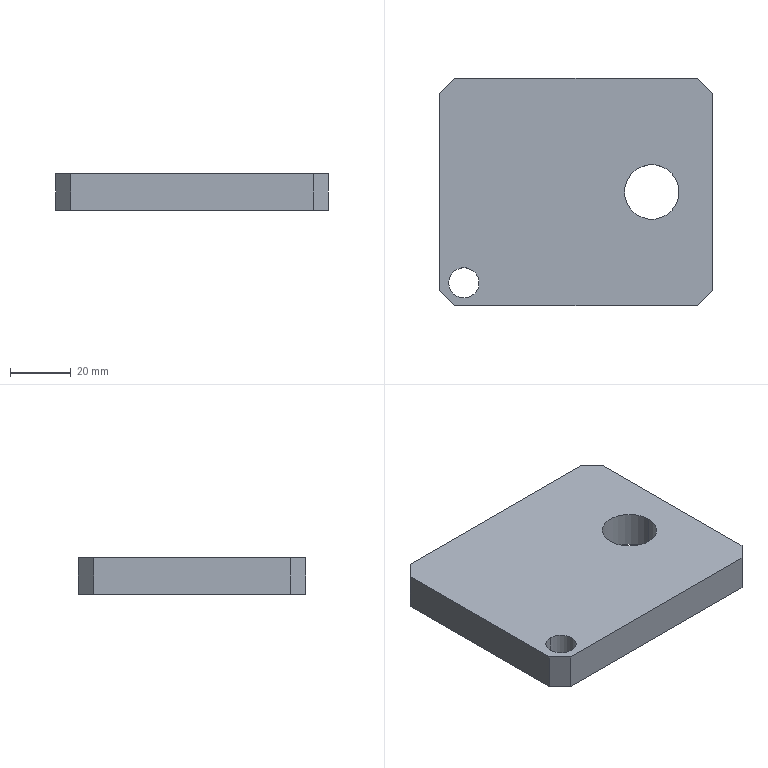Part | STEP file | [17] | 1 solid | 14 faces | box 90 x 75 x 12 mm | volume 76404 mm3 | plane 10 | cylinder 4 | commonest cylinder face diameters 10 x2 18 x2
STEP:
#1=CARTESIAN_POINT('',(79.,37.5,0.));
#2=VERTEX_POINT('',#1);
#3=CARTESIAN_POINT('',(61.,37.5,0.));
#4=VERTEX_POINT('',#3);
#5=CARTESIAN_POINT('',(70.,37.5,0.));
#6=DIRECTION('',(0.,0.,1.));
#7=DIRECTION('',(-1.,0.,0.));
#8=AXIS2_PLACEMENT_3D('',#5,#6,#7);
#9=CIRCLE('',#8,9.);
#10=EDGE_CURVE('',#2,#4,#9,.T.);
#11=ORIENTED_EDGE('',*,*,#10,.F.);
#12=CARTESIAN_POINT('',(79.,37.5,12.));
#13=VERTEX_POINT('',#12);
#14=CARTESIAN_POINT('',(79.,37.5,0.));
#15=DIRECTION('',(0.,0.,1.));
#16=VECTOR('',#15,1000.);
#17=LINE('',#14,#16);
#18=EDGE_CURVE('',#2,#13,#17,.T.);
#19=ORIENTED_EDGE('',*,*,#18,.T.);
#20=CARTESIAN_POINT('',(61.,37.5,12.));
#21=VERTEX_POINT('',#20);
#22=CARTESIAN_POINT('',(70.,37.5,12.));
#23=DIRECTION('',(0.,0.,-1.));
#24=DIRECTION('',(1.,0.,0.));
#25=AXIS2_PLACEMENT_3D('',#22,#23,#24);
#26=CIRCLE('',#25,9.);
#27=EDGE_CURVE('',#21,#13,#26,.T.);
#28=ORIENTED_EDGE('',*,*,#27,.F.);
#29=CARTESIAN_POINT('',(61.,37.5,0.));
#30=DIRECTION('',(0.,0.,1.));
#31=VECTOR('',#30,1000.);
#32=LINE('',#29,#31);
#33=EDGE_CURVE('',#4,#21,#32,.T.);
#34=ORIENTED_EDGE('',*,*,#33,.F.);
#35=EDGE_LOOP('',(#11,#19,#28,#34));
#36=FACE_OUTER_BOUND('',#35,.T.);
#37=CARTESIAN_POINT('',(70.,37.5,0.));
#38=DIRECTION('',(0.,0.,1.));
#39=DIRECTION('',(-1.,0.,0.));
#40=AXIS2_PLACEMENT_3D('',#37,#38,#39);
#41=CYLINDRICAL_SURFACE('',#40,9.);
#42=ADVANCED_FACE('',(#36),#41,.F.);
#43=CARTESIAN_POINT('',(8.,2.5,12.));
#44=VERTEX_POINT('',#43);
#45=CARTESIAN_POINT('',(8.,12.5,12.));
#46=VERTEX_POINT('',#45);
#47=CARTESIAN_POINT('',(8.,7.5,12.));
#48=DIRECTION('',(0.,0.,-1.));
#49=DIRECTION('',(0.,1.,0.));
#50=AXIS2_PLACEMENT_3D('',#47,#48,#49);
#51=CIRCLE('',#50,5.);
#52=EDGE_CURVE('',#44,#46,#51,.T.);
#53=ORIENTED_EDGE('',*,*,#52,.F.);
#54=CARTESIAN_POINT('',(8.,2.5,0.));
#55=VERTEX_POINT('',#54);
#56=CARTESIAN_POINT('',(8.,2.5,12.));
#57=DIRECTION('',(0.,0.,-1.));
#58=VECTOR('',#57,1000.);
#59=LINE('',#56,#58);
#60=EDGE_CURVE('',#44,#55,#59,.T.);
#61=ORIENTED_EDGE('',*,*,#60,.T.);
#62=CARTESIAN_POINT('',(8.,12.5,0.));
#63=VERTEX_POINT('',#62);
#64=CARTESIAN_POINT('',(8.,7.5,0.));
#65=DIRECTION('',(0.,0.,1.));
#66=DIRECTION('',(0.,-1.,0.));
#67=AXIS2_PLACEMENT_3D('',#64,#65,#66);
#68=CIRCLE('',#67,5.);
#69=EDGE_CURVE('',#63,#55,#68,.T.);
#70=ORIENTED_EDGE('',*,*,#69,.F.);
#71=CARTESIAN_POINT('',(8.,12.5,12.));
#72=DIRECTION('',(0.,0.,-1.));
#73=VECTOR('',#72,1000.);
#74=LINE('',#71,#73);
#75=EDGE_CURVE('',#46,#63,#74,.T.);
#76=ORIENTED_EDGE('',*,*,#75,.F.);
#77=EDGE_LOOP('',(#53,#61,#70,#76));
#78=FACE_OUTER_BOUND('',#77,.T.);
#79=CARTESIAN_POINT('',(8.,7.5,12.));
#80=DIRECTION('',(0.,0.,-1.));
#81=DIRECTION('',(0.,1.,0.));
#82=AXIS2_PLACEMENT_3D('',#79,#80,#81);
#83=CYLINDRICAL_SURFACE('',#82,5.);
#84=ADVANCED_FACE('',(#78),#83,.F.);
#85=CARTESIAN_POINT('',(70.,37.5,0.));
#86=DIRECTION('',(0.,0.,1.));
#87=DIRECTION('',(-1.,0.,0.));
#88=AXIS2_PLACEMENT_3D('',#85,#86,#87);
#89=CIRCLE('',#88,9.);
#90=EDGE_CURVE('',#4,#2,#89,.T.);
#91=ORIENTED_EDGE('',*,*,#90,.T.);
#92=ORIENTED_EDGE('',*,*,#10,.T.);
#93=EDGE_LOOP('',(#91,#92));
#94=FACE_BOUND('',#93,.T.);
#95=ORIENTED_EDGE('',*,*,#69,.T.);
#96=CARTESIAN_POINT('',(8.,7.5,0.));
#97=DIRECTION('',(0.,0.,1.));
#98=DIRECTION('',(0.,-1.,0.));
#99=AXIS2_PLACEMENT_3D('',#96,#97,#98);
#100=CIRCLE('',#99,5.);
#101=EDGE_CURVE('',#55,#63,#100,.T.);
#102=ORIENTED_EDGE('',*,*,#101,.T.);
#103=EDGE_LOOP('',(#95,#102));
#104=FACE_BOUND('',#103,.T.);
#105=CARTESIAN_POINT('',(85.,75.,0.));
#106=VERTEX_POINT('',#105);
#107=CARTESIAN_POINT('',(5.,75.,0.));
#108=VERTEX_POINT('',#107);
#109=CARTESIAN_POINT('',(45.,75.,0.));
#110=DIRECTION('',(-1.,0.,0.));
#111=VECTOR('',#110,1000.);
#112=LINE('',#109,#111);
#113=EDGE_CURVE('',#106,#108,#112,.T.);
#114=ORIENTED_EDGE('',*,*,#113,.F.);
#115=CARTESIAN_POINT('',(90.,70.,0.));
#116=VERTEX_POINT('',#115);
#117=CARTESIAN_POINT('',(83.75,76.25,0.));
#118=DIRECTION('',(0.7071,-0.7071,0.));
#119=VECTOR('',#118,1000.);
#120=LINE('',#117,#119);
#121=EDGE_CURVE('',#106,#116,#120,.T.);
#122=ORIENTED_EDGE('',*,*,#121,.T.);
#123=CARTESIAN_POINT('',(90.,5.,0.));
#124=VERTEX_POINT('',#123);
#125=CARTESIAN_POINT('',(90.,37.5,0.));
#126=DIRECTION('',(0.,1.,0.));
#127=VECTOR('',#126,1000.);
#128=LINE('',#125,#127);
#129=EDGE_CURVE('',#124,#116,#128,.T.);
#130=ORIENTED_EDGE('',*,*,#129,.F.);
#131=CARTESIAN_POINT('',(85.,0.,0.));
#132=VERTEX_POINT('',#131);
#133=CARTESIAN_POINT('',(83.75,-1.25,0.));
#134=DIRECTION('',(-0.7071,-0.7071,0.));
#135=VECTOR('',#134,1000.);
#136=LINE('',#133,#135);
#137=EDGE_CURVE('',#124,#132,#136,.T.);
#138=ORIENTED_EDGE('',*,*,#137,.T.);
#139=CARTESIAN_POINT('',(5.,0.,0.));
#140=VERTEX_POINT('',#139);
#141=CARTESIAN_POINT('',(45.,0.,0.));
#142=DIRECTION('',(1.,0.,0.));
#143=VECTOR('',#142,1000.);
#144=LINE('',#141,#143);
#145=EDGE_CURVE('',#140,#132,#144,.T.);
#146=ORIENTED_EDGE('',*,*,#145,.F.);
#147=CARTESIAN_POINT('',(0.,5.,0.));
#148=VERTEX_POINT('',#147);
#149=CARTESIAN_POINT('',(6.25,-1.25,0.));
#150=DIRECTION('',(-0.7071,0.7071,0.));
#151=VECTOR('',#150,1000.);
#152=LINE('',#149,#151);
#153=EDGE_CURVE('',#140,#148,#152,.T.);
#154=ORIENTED_EDGE('',*,*,#153,.T.);
#155=CARTESIAN_POINT('',(0.,70.,0.));
#156=VERTEX_POINT('',#155);
#157=CARTESIAN_POINT('',(0.,37.5,0.));
#158=DIRECTION('',(0.,-1.,0.));
#159=VECTOR('',#158,1000.);
#160=LINE('',#157,#159);
#161=EDGE_CURVE('',#156,#148,#160,.T.);
#162=ORIENTED_EDGE('',*,*,#161,.F.);
#163=CARTESIAN_POINT('',(6.25,76.25,0.));
#164=DIRECTION('',(0.7071,0.7071,0.));
#165=VECTOR('',#164,1000.);
#166=LINE('',#163,#165);
#167=EDGE_CURVE('',#156,#108,#166,.T.);
#168=ORIENTED_EDGE('',*,*,#167,.T.);
#169=EDGE_LOOP('',(#114,#122,#130,#138,#146,#154,#162,#168));
#170=FACE_OUTER_BOUND('',#169,.T.);
#171=CARTESIAN_POINT('',(45.,37.5,0.));
#172=DIRECTION('',(0.,0.,-1.));
#173=DIRECTION('',(0.,1.,0.));
#174=AXIS2_PLACEMENT_3D('',#171,#172,#173);
#175=PLANE('',#174);
#176=ADVANCED_FACE('',(#94,#104,#170),#175,.T.);
#177=CARTESIAN_POINT('',(0.,5.,12.));
#178=VERTEX_POINT('',#177);
#179=CARTESIAN_POINT('',(0.,70.,12.));
#180=VERTEX_POINT('',#179);
#181=CARTESIAN_POINT('',(0.,37.5,12.));
#182=DIRECTION('',(0.,1.,0.));
#183=VECTOR('',#182,1000.);
#184=LINE('',#181,#183);
#185=EDGE_CURVE('',#178,#180,#184,.T.);
#186=ORIENTED_EDGE('',*,*,#185,.T.);
#187=CARTESIAN_POINT('',(0.,70.,12.));
#188=DIRECTION('',(0.,0.,-1.));
#189=VECTOR('',#188,1000.);
#190=LINE('',#187,#189);
#191=EDGE_CURVE('',#180,#156,#190,.T.);
#192=ORIENTED_EDGE('',*,*,#191,.T.);
#193=ORIENTED_EDGE('',*,*,#161,.T.);
#194=CARTESIAN_POINT('',(0.,5.,12.));
#195=DIRECTION('',(0.,0.,1.));
#196=VECTOR('',#195,1000.);
#197=LINE('',#194,#196);
#198=EDGE_CURVE('',#148,#178,#197,.T.);
#199=ORIENTED_EDGE('',*,*,#198,.T.);
#200=EDGE_LOOP('',(#186,#192,#193,#199));
#201=FACE_OUTER_BOUND('',#200,.T.);
#202=CARTESIAN_POINT('',(0.,37.5,12.));
#203=DIRECTION('',(-1.,0.,0.));
#204=DIRECTION('',(0.,0.,1.));
#205=AXIS2_PLACEMENT_3D('',#202,#203,#204);
#206=PLANE('',#205);
#207=ADVANCED_FACE('',(#201),#206,.T.);
#208=ORIENTED_EDGE('',*,*,#145,.T.);
#209=CARTESIAN_POINT('',(85.,0.,12.));
#210=VERTEX_POINT('',#209);
#211=CARTESIAN_POINT('',(85.,0.,12.));
#212=DIRECTION('',(0.,0.,1.));
#213=VECTOR('',#212,1000.);
#214=LINE('',#211,#213);
#215=EDGE_CURVE('',#132,#210,#214,.T.);
#216=ORIENTED_EDGE('',*,*,#215,.T.);
#217=CARTESIAN_POINT('',(5.,0.,12.));
#218=VERTEX_POINT('',#217);
#219=CARTESIAN_POINT('',(45.,0.,12.));
#220=DIRECTION('',(-1.,0.,0.));
#221=VECTOR('',#220,1000.);
#222=LINE('',#219,#221);
#223=EDGE_CURVE('',#210,#218,#222,.T.);
#224=ORIENTED_EDGE('',*,*,#223,.T.);
#225=CARTESIAN_POINT('',(5.,0.,12.));
#226=DIRECTION('',(0.,0.,-1.));
#227=VECTOR('',#226,1000.);
#228=LINE('',#225,#227);
#229=EDGE_CURVE('',#218,#140,#228,.T.);
#230=ORIENTED_EDGE('',*,*,#229,.T.);
#231=EDGE_LOOP('',(#208,#216,#224,#230));
#232=FACE_OUTER_BOUND('',#231,.T.);
#233=CARTESIAN_POINT('',(45.,0.,12.));
#234=DIRECTION('',(0.,-1.,0.));
#235=DIRECTION('',(0.,0.,-1.));
#236=AXIS2_PLACEMENT_3D('',#233,#234,#235);
#237=PLANE('',#236);
#238=ADVANCED_FACE('',(#232),#237,.T.);
#239=ORIENTED_EDGE('',*,*,#129,.T.);
#240=CARTESIAN_POINT('',(90.,70.,12.));
#241=VERTEX_POINT('',#240);
#242=CARTESIAN_POINT('',(90.,70.,12.));
#243=DIRECTION('',(0.,0.,1.));
#244=VECTOR('',#243,1000.);
#245=LINE('',#242,#244);
#246=EDGE_CURVE('',#116,#241,#245,.T.);
#247=ORIENTED_EDGE('',*,*,#246,.T.);
#248=CARTESIAN_POINT('',(90.,5.,12.));
#249=VERTEX_POINT('',#248);
#250=CARTESIAN_POINT('',(90.,37.5,12.));
#251=DIRECTION('',(0.,-1.,0.));
#252=VECTOR('',#251,1000.);
#253=LINE('',#250,#252);
#254=EDGE_CURVE('',#241,#249,#253,.T.);
#255=ORIENTED_EDGE('',*,*,#254,.T.);
#256=CARTESIAN_POINT('',(90.,5.,12.));
#257=DIRECTION('',(0.,0.,-1.));
#258=VECTOR('',#257,1000.);
#259=LINE('',#256,#258);
#260=EDGE_CURVE('',#249,#124,#259,.T.);
#261=ORIENTED_EDGE('',*,*,#260,.T.);
#262=EDGE_LOOP('',(#239,#247,#255,#261));
#263=FACE_OUTER_BOUND('',#262,.T.);
#264=CARTESIAN_POINT('',(90.,37.5,12.));
#265=DIRECTION('',(1.,0.,0.));
#266=DIRECTION('',(0.,0.,-1.));
#267=AXIS2_PLACEMENT_3D('',#264,#265,#266);
#268=PLANE('',#267);
#269=ADVANCED_FACE('',(#263),#268,.T.);
#270=ORIENTED_EDGE('',*,*,#27,.T.);
#271=CARTESIAN_POINT('',(70.,37.5,12.));
#272=DIRECTION('',(0.,0.,-1.));
#273=DIRECTION('',(1.,0.,0.));
#274=AXIS2_PLACEMENT_3D('',#271,#272,#273);
#275=CIRCLE('',#274,9.);
#276=EDGE_CURVE('',#13,#21,#275,.T.);
#277=ORIENTED_EDGE('',*,*,#276,.T.);
#278=EDGE_LOOP('',(#270,#277));
#279=FACE_BOUND('',#278,.T.);
#280=CARTESIAN_POINT('',(8.,7.5,12.));
#281=DIRECTION('',(0.,0.,-1.));
#282=DIRECTION('',(0.,1.,0.));
#283=AXIS2_PLACEMENT_3D('',#280,#281,#282);
#284=CIRCLE('',#283,5.);
#285=EDGE_CURVE('',#46,#44,#284,.T.);
#286=ORIENTED_EDGE('',*,*,#285,.T.);
#287=ORIENTED_EDGE('',*,*,#52,.T.);
#288=EDGE_LOOP('',(#286,#287));
#289=FACE_BOUND('',#288,.T.);
#290=ORIENTED_EDGE('',*,*,#254,.F.);
#291=CARTESIAN_POINT('',(85.,75.,12.));
#292=VERTEX_POINT('',#291);
#293=CARTESIAN_POINT('',(83.75,76.25,12.));
#294=DIRECTION('',(-0.7071,0.7071,0.));
#295=VECTOR('',#294,1000.);
#296=LINE('',#293,#295);
#297=EDGE_CURVE('',#241,#292,#296,.T.);
#298=ORIENTED_EDGE('',*,*,#297,.T.);
#299=CARTESIAN_POINT('',(5.,75.,12.));
#300=VERTEX_POINT('',#299);
#301=CARTESIAN_POINT('',(45.,75.,12.));
#302=DIRECTION('',(1.,0.,0.));
#303=VECTOR('',#302,1000.);
#304=LINE('',#301,#303);
#305=EDGE_CURVE('',#300,#292,#304,.T.);
#306=ORIENTED_EDGE('',*,*,#305,.F.);
#307=CARTESIAN_POINT('',(6.25,76.25,12.));
#308=DIRECTION('',(-0.7071,-0.7071,0.));
#309=VECTOR('',#308,1000.);
#310=LINE('',#307,#309);
#311=EDGE_CURVE('',#300,#180,#310,.T.);
#312=ORIENTED_EDGE('',*,*,#311,.T.);
#313=ORIENTED_EDGE('',*,*,#185,.F.);
#314=CARTESIAN_POINT('',(6.25,-1.25,12.));
#315=DIRECTION('',(0.7071,-0.7071,0.));
#316=VECTOR('',#315,1000.);
#317=LINE('',#314,#316);
#318=EDGE_CURVE('',#178,#218,#317,.T.);
#319=ORIENTED_EDGE('',*,*,#318,.T.);
#320=ORIENTED_EDGE('',*,*,#223,.F.);
#321=CARTESIAN_POINT('',(83.75,-1.25,12.));
#322=DIRECTION('',(0.7071,0.7071,0.));
#323=VECTOR('',#322,1000.);
#324=LINE('',#321,#323);
#325=EDGE_CURVE('',#210,#249,#324,.T.);
#326=ORIENTED_EDGE('',*,*,#325,.T.);
#327=EDGE_LOOP('',(#290,#298,#306,#312,#313,#319,#320,#326));
#328=FACE_OUTER_BOUND('',#327,.T.);
#329=CARTESIAN_POINT('',(45.,37.5,12.));
#330=DIRECTION('',(0.,0.,1.));
#331=DIRECTION('',(0.,-1.,0.));
#332=AXIS2_PLACEMENT_3D('',#329,#330,#331);
#333=PLANE('',#332);
#334=ADVANCED_FACE('',(#279,#289,#328),#333,.T.);
#335=ORIENTED_EDGE('',*,*,#305,.T.);
#336=CARTESIAN_POINT('',(85.,75.,12.));
#337=DIRECTION('',(0.,0.,-1.));
#338=VECTOR('',#337,1000.);
#339=LINE('',#336,#338);
#340=EDGE_CURVE('',#292,#106,#339,.T.);
#341=ORIENTED_EDGE('',*,*,#340,.T.);
#342=ORIENTED_EDGE('',*,*,#113,.T.);
#343=CARTESIAN_POINT('',(5.,75.,12.));
#344=DIRECTION('',(0.,0.,1.));
#345=VECTOR('',#344,1000.);
#346=LINE('',#343,#345);
#347=EDGE_CURVE('',#108,#300,#346,.T.);
#348=ORIENTED_EDGE('',*,*,#347,.T.);
#349=EDGE_LOOP('',(#335,#341,#342,#348));
#350=FACE_OUTER_BOUND('',#349,.T.);
#351=CARTESIAN_POINT('',(45.,75.,12.));
#352=DIRECTION('',(0.,1.,0.));
#353=DIRECTION('',(0.,0.,1.));
#354=AXIS2_PLACEMENT_3D('',#351,#352,#353);
#355=PLANE('',#354);
#356=ADVANCED_FACE('',(#350),#355,.T.);
#357=ORIENTED_EDGE('',*,*,#311,.F.);
#358=ORIENTED_EDGE('',*,*,#347,.F.);
#359=ORIENTED_EDGE('',*,*,#167,.F.);
#360=ORIENTED_EDGE('',*,*,#191,.F.);
#361=EDGE_LOOP('',(#357,#358,#359,#360));
#362=FACE_OUTER_BOUND('',#361,.T.);
#363=CARTESIAN_POINT('',(0.,70.,12.));
#364=DIRECTION('',(0.7071,-0.7071,0.));
#365=DIRECTION('',(0.,0.,-1.));
#366=AXIS2_PLACEMENT_3D('',#363,#364,#365);
#367=PLANE('',#366);
#368=ADVANCED_FACE('',(#362),#367,.F.);
#369=ORIENTED_EDGE('',*,*,#318,.F.);
#370=ORIENTED_EDGE('',*,*,#198,.F.);
#371=ORIENTED_EDGE('',*,*,#153,.F.);
#372=ORIENTED_EDGE('',*,*,#229,.F.);
#373=EDGE_LOOP('',(#369,#370,#371,#372));
#374=FACE_OUTER_BOUND('',#373,.T.);
#375=CARTESIAN_POINT('',(5.,0.,12.));
#376=DIRECTION('',(0.7071,0.7071,0.));
#377=DIRECTION('',(0.,0.,-1.));
#378=AXIS2_PLACEMENT_3D('',#375,#376,#377);
#379=PLANE('',#378);
#380=ADVANCED_FACE('',(#374),#379,.F.);
#381=ORIENTED_EDGE('',*,*,#297,.F.);
#382=ORIENTED_EDGE('',*,*,#246,.F.);
#383=ORIENTED_EDGE('',*,*,#121,.F.);
#384=ORIENTED_EDGE('',*,*,#340,.F.);
#385=EDGE_LOOP('',(#381,#382,#383,#384));
#386=FACE_OUTER_BOUND('',#385,.T.);
#387=CARTESIAN_POINT('',(85.,75.,12.));
#388=DIRECTION('',(-0.7071,-0.7071,0.));
#389=DIRECTION('',(0.,0.,-1.));
#390=AXIS2_PLACEMENT_3D('',#387,#388,#389);
#391=PLANE('',#390);
#392=ADVANCED_FACE('',(#386),#391,.F.);
#393=ORIENTED_EDGE('',*,*,#325,.F.);
#394=ORIENTED_EDGE('',*,*,#215,.F.);
#395=ORIENTED_EDGE('',*,*,#137,.F.);
#396=ORIENTED_EDGE('',*,*,#260,.F.);
#397=EDGE_LOOP('',(#393,#394,#395,#396));
#398=FACE_OUTER_BOUND('',#397,.T.);
#399=CARTESIAN_POINT('',(90.,5.,12.));
#400=DIRECTION('',(-0.7071,0.7071,0.));
#401=DIRECTION('',(0.,0.,-1.));
#402=AXIS2_PLACEMENT_3D('',#399,#400,#401);
#403=PLANE('',#402);
#404=ADVANCED_FACE('',(#398),#403,.F.);
#405=ORIENTED_EDGE('',*,*,#60,.F.);
#406=ORIENTED_EDGE('',*,*,#285,.F.);
#407=ORIENTED_EDGE('',*,*,#75,.T.);
#408=ORIENTED_EDGE('',*,*,#101,.F.);
#409=EDGE_LOOP('',(#405,#406,#407,#408));
#410=FACE_OUTER_BOUND('',#409,.T.);
#411=CARTESIAN_POINT('',(8.,7.5,12.));
#412=DIRECTION('',(0.,0.,-1.));
#413=DIRECTION('',(0.,1.,0.));
#414=AXIS2_PLACEMENT_3D('',#411,#412,#413);
#415=CYLINDRICAL_SURFACE('',#414,5.);
#416=ADVANCED_FACE('',(#410),#415,.F.);
#417=ORIENTED_EDGE('',*,*,#18,.F.);
#418=ORIENTED_EDGE('',*,*,#90,.F.);
#419=ORIENTED_EDGE('',*,*,#33,.T.);
#420=ORIENTED_EDGE('',*,*,#276,.F.);
#421=EDGE_LOOP('',(#417,#418,#419,#420));
#422=FACE_OUTER_BOUND('',#421,.T.);
#423=CARTESIAN_POINT('',(70.,37.5,0.));
#424=DIRECTION('',(0.,0.,1.));
#425=DIRECTION('',(-1.,0.,0.));
#426=AXIS2_PLACEMENT_3D('',#423,#424,#425);
#427=CYLINDRICAL_SURFACE('',#426,9.);
#428=ADVANCED_FACE('',(#422),#427,.F.);
#429=CLOSED_SHELL('',(#42,#84,#176,#207,#238,#269,#334,#356,#368,#380,#392,#404,#416,#428));
#430=MANIFOLD_SOLID_BREP('',#429);
#431=CARTESIAN_POINT('',(0.,0.,0.));
#432=DIRECTION('',(0.,0.,1.));
#433=DIRECTION('',(1.,0.,0.));
#434=AXIS2_PLACEMENT_3D('',#431,#432,#433);
#435=(LENGTH_UNIT()NAMED_UNIT(*)SI_UNIT(.MILLI.,.METRE.));
#436=UNCERTAINTY_MEASURE_WITH_UNIT(LENGTH_MEASURE(0.00001),#435,'','');
#437=(NAMED_UNIT(*)PLANE_ANGLE_UNIT()SI_UNIT($,.RADIAN.));
#438=(NAMED_UNIT(*)SI_UNIT($,.STERADIAN.)SOLID_ANGLE_UNIT());
#439=(GEOMETRIC_REPRESENTATION_CONTEXT(3)GLOBAL_UNCERTAINTY_ASSIGNED_CONTEXT((#436))GLOBAL_UNIT_ASSIGNED_CONTEXT((#435,#437,#438))REPRESENTATION_CONTEXT('',''));
#440=ADVANCED_BREP_SHAPE_REPRESENTATION('',(#430,#434),#439);